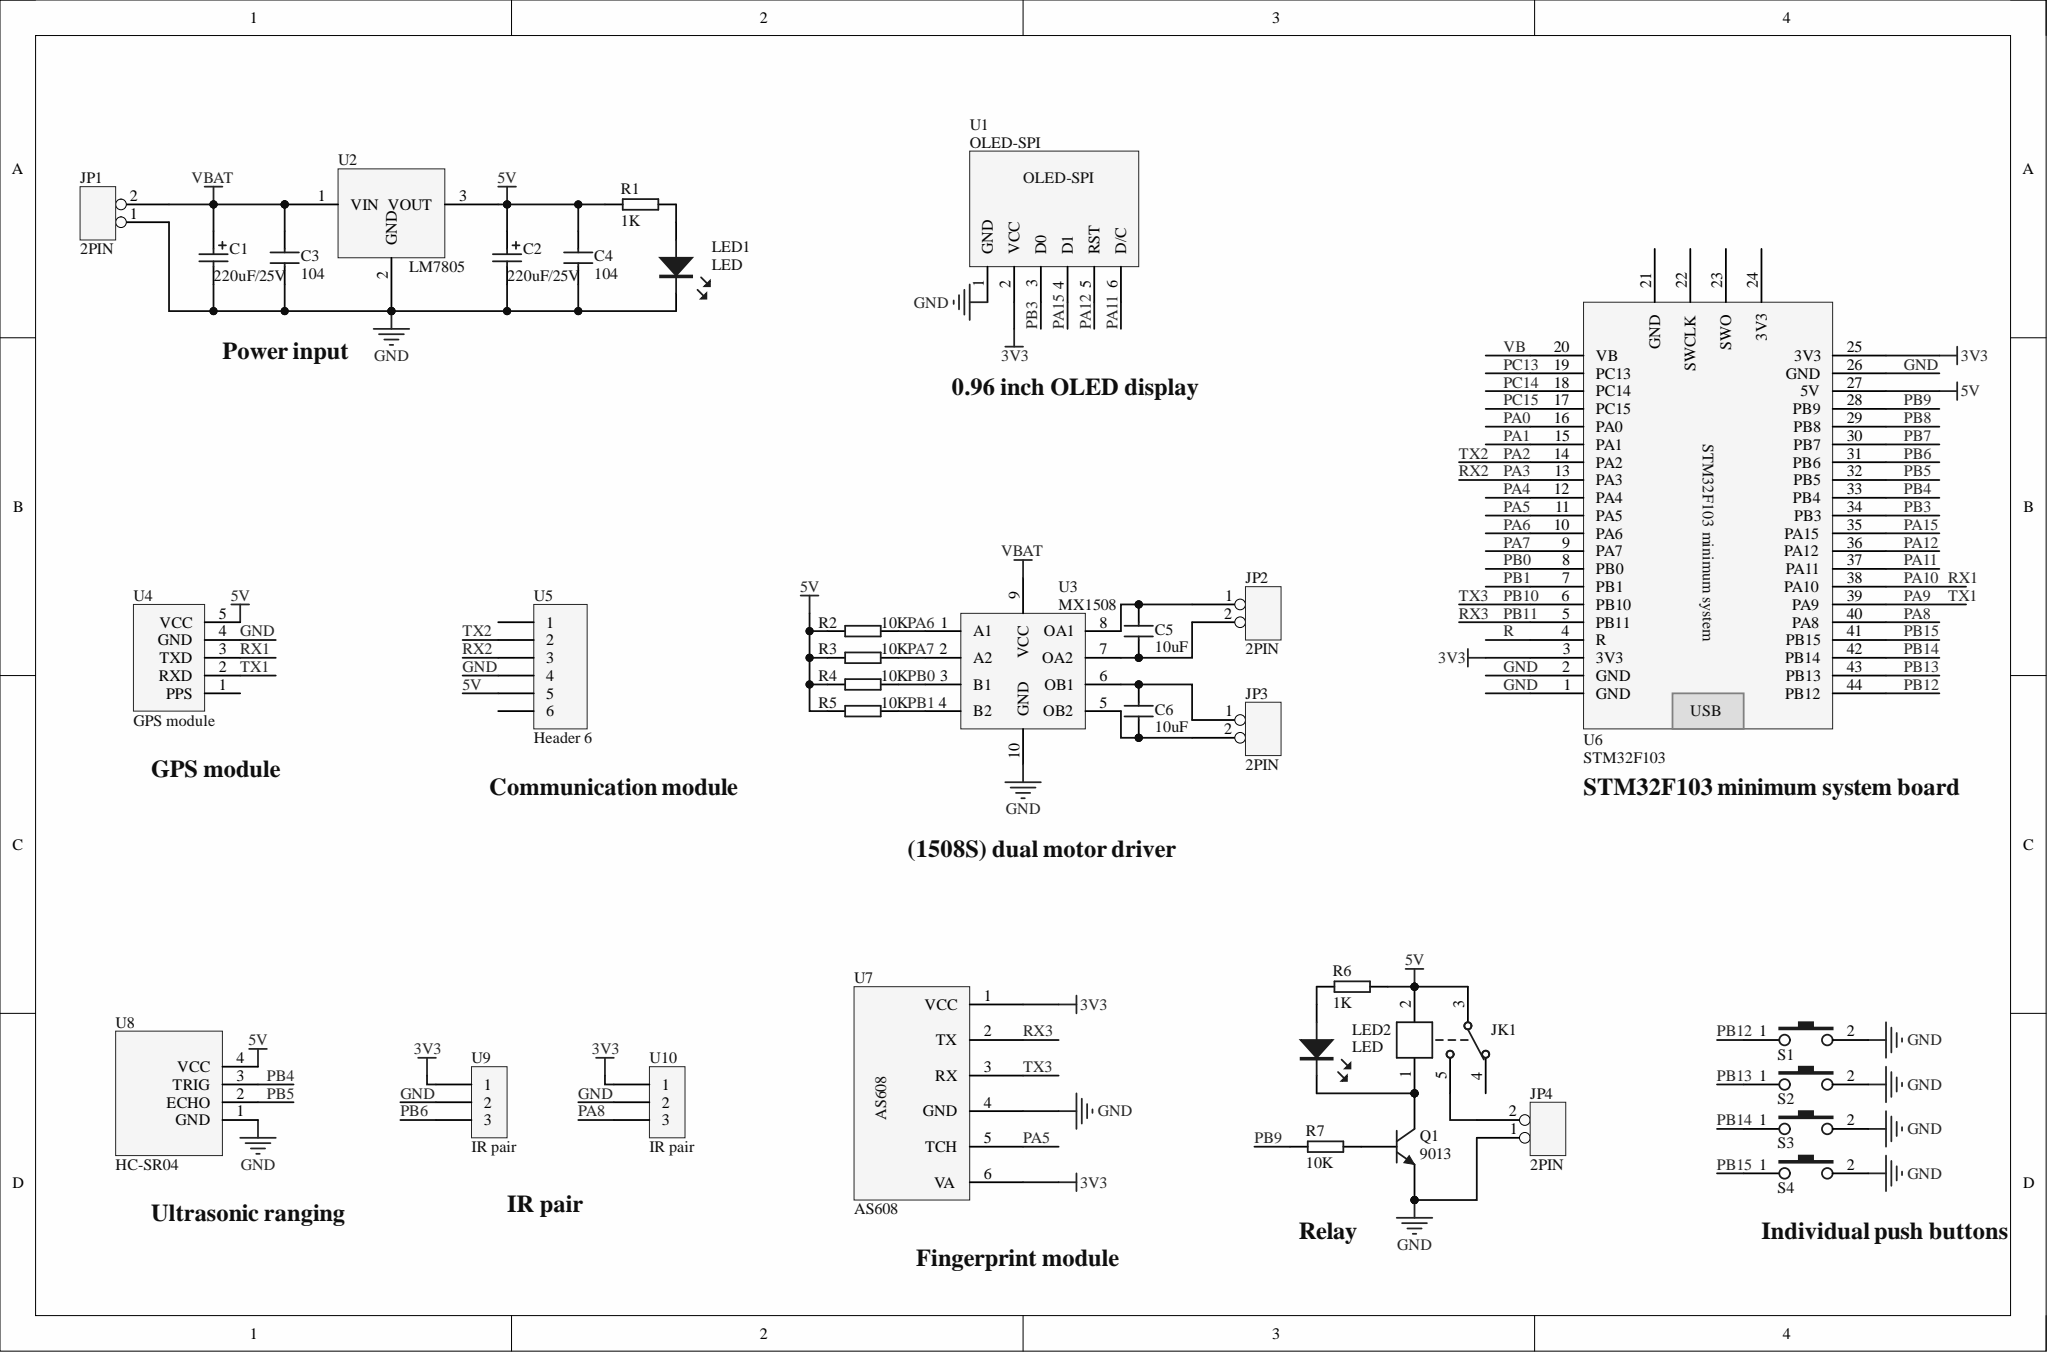Circuit board | Altium Designer | 35 parts | 37 nets
Bill of materials:
Comment,Description,Designator,Footprint,LibRef,Quantity
"220uF/25V","Polarized Capacitor (Axial)","C1, C2","DIP-EC3.5X8X11.5","Cap Pol2","2"
"104","non-polarized capacitor","C3, C4","RAD-0.2","CAP","2"
"10uF","non-polarized capacitor","C5, C6","0603C","CAP","2"
"SRD-05VDC-SL-C","5V single-group converter","JK1","SRD-C_B","SRD-05VDC-SL-C","1"
"2PIN","","JP1, JP2, JP3, JP4","XH2.54-LI-2P","2PIN","4"
"LED","","LED1, LED2","LED 3MM-B","LED","2"
"9013","NPN General Purpose Amplifier","Q1","TO-92A","2N3904","1"
"1K","resistor","R1, R6","AXIAL0.3","RES","2"
"10K","resistor","R2, R3, R4, R5, R7","AXIAL0.3","RES","5"
"BUTTOM","push button","S1, S2, S3, S4","DIP-6X6X5","BUTTOM","4"
"OLED-SPI","OLED-SPI","U1","OLED-SPI","OLED-SPI","1"
"LM7805","","U2","TO220A","LM7805","1"
"MX1508","Motor driver module","U3","马达驱动芯片","马达驱动模块","1"
"GPS module","","U4","GPS","GPS","1"
"Header 6","Header, 6-Pin","U5","Pin HDR1X6/2.54mm-S","Header 6","1"
"STM32F103","STM32F103","U6","STM32FF103","STM32F103","1"
"AS608","AS608","U7","AS608","指纹模块","1"
"HC-SR04","Ultrasonic module","U8","超声波MODE","超声波MODE","1"
"IR pair","","U9, U10","火焰传感器","Pin HDR1X3","2"
Netlist (Protel format):
[
C1
DIP-EC3.5X8X11.5
220uF/25V



]
[
C2
DIP-EC3.5X8X11.5
220uF/25V



]
[
C3
RAD-0.2
104



]
[
C4
RAD-0.2
104



]
[
C5
0603C
10uF



]
[
C6
0603C
10uF



]
[
JK1
SRD-C_B
SRD-05VDC-SL-C



]
[
JP1
XH2.54-LI-2P
2PIN



]
[
JP2
XH2.54-LI-2P
2PIN



]
[
JP3
XH2.54-LI-2P
2PIN



]
[
JP4
XH2.54-LI-2P
2PIN



]
[
LED1
LED 3MM-B
LED



]
[
LED2
LED 3MM-B
LED



]
[
Q1
TO-92A
9013



]
[
R1
AXIAL0.3
1K



]
[
R2
AXIAL0.3
10K



]
[
R3
AXIAL0.3
10K



]
[
R4
AXIAL0.3
10K



]
[
R5
AXIAL0.3
10K



]
[
R6
AXIAL0.3
1K



]
[
R7
AXIAL0.3
10K



]
[
S1
DIP-6X6X5
BUTTOM



]
[
S2
DIP-6X6X5
BUTTOM



]
[
S3
DIP-6X6X5
BUTTOM



]
[
S4
DIP-6X6X5
BUTTOM



]
[
U1
OLED-SPI
OLED-SPI



]
[
U2
TO220A
LM7805



]
[
U3
马达驱动芯片
MX1508



]
[
U4
GPS
GPS module



]
[
U5
Pin HDR1X6/2.54mm-S
Header 6



]
[
U6
STM32FF103
STM32F103



]
[
U7
AS608
AS608



]
[
U8
超声波MODE
HC-SR04



]
[
U9
火焰传感器
IR pair



]
[
U10
火焰传感器
IR pair



]
(
VBAT
C1-1
C3-2
JP1-2
U2-1
U3-9
)
(
PB15
S4-1
U6-41
)
(
PB14
S3-1
U6-42
)
(
PB13
S2-1
U6-43
)
(
PB12
S1-1
U6-44
)
(
PB11
U6-5
U7-2
)
(
PB10
U6-6
U7-3
)
(
PB9
R7-1
U6-28
)
(
PB6
U6-31
U9-3
)
(
PB5
U6-32
U8-2
)
(
PB4
U6-33
U8-3
)
(
PB3
U1-3
U6-34
)
(
PB1
R5-2
U3-4
U6-7
)
(
PB0
R4-2
U3-3
U6-8
)
(
PA15
U1-4
U6-35
)
(
PA12
U1-5
U6-36
)
(
PA11
U1-6
U6-37
)
(
PA10
U4-3
U6-38
)
(
PA9
U4-2
U6-39
)
(
PA8
U6-40
U10-3
)
(
PA7
R3-2
U3-2
U6-9
)
(
PA6
R2-2
U3-1
U6-10
)
(
PA5
U6-11
U7-5
)
(
PA3
U5-3
U6-13
)
(
PA2
U5-2
U6-14
)
(
NetQ1_B
Q1-B
R7-2
)
(
NetLED2_1
LED2-1
R6-1
)
(
NetLED1_1
LED1-1
R1-1
)
(
NetJK1_5
JK1-5
JP4-2
)
(
NetJK1_1
JK1-1
LED2-2
Q1-C
)
(
NetC6_2
C6-2
JP3-1
U3-6
)
(
NetC6_1
C6-1
JP3-2
U3-5
)
(
NetC5_2
C5-2
JP2-1
U3-8
)
(
NetC5_1
C5-1
JP2-2
U3-7
)
(
GND
C1-2
C2-2
C3-1
C4-1
JP1-1
JP4-1
LED1-2
Q1-E
S1-2
S2-2
S3-2
S4-2
U1-1
U2-2
U3-10
U4-4
U5-4
U6-1
U6-2
U6-26
U7-4
U8-1
U9-2
U10-2
)
(
5V
C2-1
C4-2
JK1-2
JK1-3
R1-2
R2-1
R3-1
R4-1
R5-1
R6-2
U2-3
U4-5
U5-5
U6-27
U8-4
)
(
3V3
U1-2
U6-3
U6-25
U7-1
U7-6
U9-1
U10-1
)